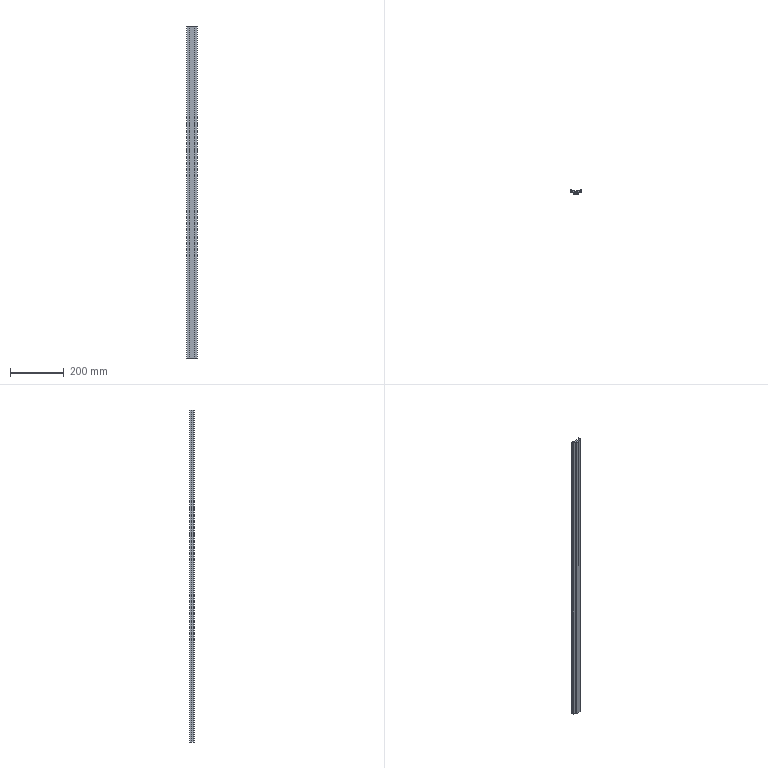Part | SolidWorks | features BaseBody 1 | 1 solid | 18 faces | box 38 x 15 x 1230 mm | volume 313896 mm3 | plane 18
STEP:
#1=CARTESIAN_POINT('',(-16.,11.5,1230.));
#2=VERTEX_POINT('',#1);
#3=CARTESIAN_POINT('',(-16.,11.5,0.));
#4=VERTEX_POINT('',#3);
#5=CARTESIAN_POINT('',(-16.,11.5,1230.));
#6=DIRECTION('',(0.,0.,-1.));
#7=VECTOR('',#6,1000.);
#8=LINE('',#5,#7);
#9=EDGE_CURVE('',#2,#4,#8,.T.);
#10=ORIENTED_EDGE('',*,*,#9,.F.);
#11=CARTESIAN_POINT('',(16.,11.5,1230.));
#12=VERTEX_POINT('',#11);
#13=CARTESIAN_POINT('',(16.,11.5,1230.));
#14=DIRECTION('',(-1.,0.,0.));
#15=VECTOR('',#14,1000.);
#16=LINE('',#13,#15);
#17=EDGE_CURVE('',#12,#2,#16,.T.);
#18=ORIENTED_EDGE('',*,*,#17,.F.);
#19=CARTESIAN_POINT('',(16.,11.5,0.));
#20=VERTEX_POINT('',#19);
#21=CARTESIAN_POINT('',(16.,11.5,1230.));
#22=DIRECTION('',(0.,0.,1.));
#23=VECTOR('',#22,1000.);
#24=LINE('',#21,#23);
#25=EDGE_CURVE('',#20,#12,#24,.T.);
#26=ORIENTED_EDGE('',*,*,#25,.F.);
#27=CARTESIAN_POINT('',(16.,11.5,0.));
#28=DIRECTION('',(1.,0.,0.));
#29=VECTOR('',#28,1000.);
#30=LINE('',#27,#29);
#31=EDGE_CURVE('',#4,#20,#30,.T.);
#32=ORIENTED_EDGE('',*,*,#31,.F.);
#33=EDGE_LOOP('',(#10,#18,#26,#32));
#34=FACE_OUTER_BOUND('',#33,.T.);
#35=CARTESIAN_POINT('',(16.,11.5,1230.));
#36=DIRECTION('',(0.,-1.,0.));
#37=DIRECTION('',(1.,0.,0.));
#38=AXIS2_PLACEMENT_3D('',#35,#36,#37);
#39=PLANE('',#38);
#40=ADVANCED_FACE('',(#34),#39,.F.);
#41=CARTESIAN_POINT('',(-3.5,3.,0.));
#42=VERTEX_POINT('',#41);
#43=CARTESIAN_POINT('',(-10.,3.,0.));
#44=VERTEX_POINT('',#43);
#45=CARTESIAN_POINT('',(0.,3.,0.));
#46=DIRECTION('',(-1.,0.,0.));
#47=VECTOR('',#46,1000.);
#48=LINE('',#45,#47);
#49=EDGE_CURVE('',#42,#44,#48,.T.);
#50=ORIENTED_EDGE('',*,*,#49,.F.);
#51=CARTESIAN_POINT('',(-3.5,7.8,0.));
#52=VERTEX_POINT('',#51);
#53=CARTESIAN_POINT('',(-3.5,0.,0.));
#54=DIRECTION('',(0.,-1.,0.));
#55=VECTOR('',#54,1000.);
#56=LINE('',#53,#55);
#57=EDGE_CURVE('',#52,#42,#56,.T.);
#58=ORIENTED_EDGE('',*,*,#57,.F.);
#59=CARTESIAN_POINT('',(-19.,7.8,0.));
#60=VERTEX_POINT('',#59);
#61=CARTESIAN_POINT('',(0.,7.8,0.));
#62=DIRECTION('',(1.,0.,0.));
#63=VECTOR('',#62,1000.);
#64=LINE('',#61,#63);
#65=EDGE_CURVE('',#60,#52,#64,.T.);
#66=ORIENTED_EDGE('',*,*,#65,.F.);
#67=CARTESIAN_POINT('',(-19.,15.,0.));
#68=VERTEX_POINT('',#67);
#69=CARTESIAN_POINT('',(-19.,0.,0.));
#70=DIRECTION('',(0.,-1.,0.));
#71=VECTOR('',#70,1000.);
#72=LINE('',#69,#71);
#73=EDGE_CURVE('',#68,#60,#72,.T.);
#74=ORIENTED_EDGE('',*,*,#73,.F.);
#75=CARTESIAN_POINT('',(-16.,15.,0.));
#76=VERTEX_POINT('',#75);
#77=CARTESIAN_POINT('',(0.,15.,0.));
#78=DIRECTION('',(-1.,0.,0.));
#79=VECTOR('',#78,1000.);
#80=LINE('',#77,#79);
#81=EDGE_CURVE('',#76,#68,#80,.T.);
#82=ORIENTED_EDGE('',*,*,#81,.F.);
#83=CARTESIAN_POINT('',(-16.,0.,0.));
#84=DIRECTION('',(0.,1.,0.));
#85=VECTOR('',#84,1000.);
#86=LINE('',#83,#85);
#87=EDGE_CURVE('',#4,#76,#86,.T.);
#88=ORIENTED_EDGE('',*,*,#87,.F.);
#89=ORIENTED_EDGE('',*,*,#31,.T.);
#90=CARTESIAN_POINT('',(16.,15.,0.));
#91=VERTEX_POINT('',#90);
#92=CARTESIAN_POINT('',(16.,0.,0.));
#93=DIRECTION('',(0.,-1.,0.));
#94=VECTOR('',#93,1000.);
#95=LINE('',#92,#94);
#96=EDGE_CURVE('',#91,#20,#95,.T.);
#97=ORIENTED_EDGE('',*,*,#96,.F.);
#98=CARTESIAN_POINT('',(19.,15.,0.));
#99=VERTEX_POINT('',#98);
#100=CARTESIAN_POINT('',(0.,15.,0.));
#101=DIRECTION('',(-1.,0.,0.));
#102=VECTOR('',#101,1000.);
#103=LINE('',#100,#102);
#104=EDGE_CURVE('',#99,#91,#103,.T.);
#105=ORIENTED_EDGE('',*,*,#104,.F.);
#106=CARTESIAN_POINT('',(19.,7.8,0.));
#107=VERTEX_POINT('',#106);
#108=CARTESIAN_POINT('',(19.,0.,0.));
#109=DIRECTION('',(0.,1.,0.));
#110=VECTOR('',#109,1000.);
#111=LINE('',#108,#110);
#112=EDGE_CURVE('',#107,#99,#111,.T.);
#113=ORIENTED_EDGE('',*,*,#112,.F.);
#114=CARTESIAN_POINT('',(3.5,7.8,0.));
#115=VERTEX_POINT('',#114);
#116=CARTESIAN_POINT('',(0.,7.8,0.));
#117=DIRECTION('',(1.,0.,0.));
#118=VECTOR('',#117,1000.);
#119=LINE('',#116,#118);
#120=EDGE_CURVE('',#115,#107,#119,.T.);
#121=ORIENTED_EDGE('',*,*,#120,.F.);
#122=CARTESIAN_POINT('',(3.5,3.,0.));
#123=VERTEX_POINT('',#122);
#124=CARTESIAN_POINT('',(3.5,0.,0.));
#125=DIRECTION('',(0.,1.,0.));
#126=VECTOR('',#125,1000.);
#127=LINE('',#124,#126);
#128=EDGE_CURVE('',#123,#115,#127,.T.);
#129=ORIENTED_EDGE('',*,*,#128,.F.);
#130=CARTESIAN_POINT('',(10.,3.,0.));
#131=VERTEX_POINT('',#130);
#132=CARTESIAN_POINT('',(0.,3.,0.));
#133=DIRECTION('',(-1.,0.,0.));
#134=VECTOR('',#133,1000.);
#135=LINE('',#132,#134);
#136=EDGE_CURVE('',#131,#123,#135,.T.);
#137=ORIENTED_EDGE('',*,*,#136,.F.);
#138=CARTESIAN_POINT('',(10.,0.,0.));
#139=VERTEX_POINT('',#138);
#140=CARTESIAN_POINT('',(10.,0.,0.));
#141=DIRECTION('',(0.,1.,0.));
#142=VECTOR('',#141,1000.);
#143=LINE('',#140,#142);
#144=EDGE_CURVE('',#139,#131,#143,.T.);
#145=ORIENTED_EDGE('',*,*,#144,.F.);
#146=CARTESIAN_POINT('',(-10.,0.,0.));
#147=VERTEX_POINT('',#146);
#148=CARTESIAN_POINT('',(0.,0.,0.));
#149=DIRECTION('',(1.,0.,0.));
#150=VECTOR('',#149,1000.);
#151=LINE('',#148,#150);
#152=EDGE_CURVE('',#147,#139,#151,.T.);
#153=ORIENTED_EDGE('',*,*,#152,.F.);
#154=CARTESIAN_POINT('',(-10.,0.,0.));
#155=DIRECTION('',(0.,-1.,0.));
#156=VECTOR('',#155,1000.);
#157=LINE('',#154,#156);
#158=EDGE_CURVE('',#44,#147,#157,.T.);
#159=ORIENTED_EDGE('',*,*,#158,.F.);
#160=EDGE_LOOP('',(#50,#58,#66,#74,#82,#88,#89,#97,#105,#113,#121,#129,#137,#145,#153,#159));
#161=FACE_OUTER_BOUND('',#160,.T.);
#162=CARTESIAN_POINT('',(0.,0.,0.));
#163=DIRECTION('',(0.,0.,1.));
#164=DIRECTION('',(1.,0.,0.));
#165=AXIS2_PLACEMENT_3D('',#162,#163,#164);
#166=PLANE('',#165);
#167=ADVANCED_FACE('',(#161),#166,.F.);
#168=CARTESIAN_POINT('',(-16.,15.,1230.));
#169=VERTEX_POINT('',#168);
#170=CARTESIAN_POINT('',(-16.,15.,1230.));
#171=DIRECTION('',(0.,0.,-1.));
#172=VECTOR('',#171,1000.);
#173=LINE('',#170,#172);
#174=EDGE_CURVE('',#169,#76,#173,.T.);
#175=ORIENTED_EDGE('',*,*,#174,.F.);
#176=CARTESIAN_POINT('',(-16.,11.5,1230.));
#177=DIRECTION('',(0.,1.,0.));
#178=VECTOR('',#177,1000.);
#179=LINE('',#176,#178);
#180=EDGE_CURVE('',#2,#169,#179,.T.);
#181=ORIENTED_EDGE('',*,*,#180,.F.);
#182=ORIENTED_EDGE('',*,*,#9,.T.);
#183=ORIENTED_EDGE('',*,*,#87,.T.);
#184=EDGE_LOOP('',(#175,#181,#182,#183));
#185=FACE_OUTER_BOUND('',#184,.T.);
#186=CARTESIAN_POINT('',(-16.,11.5,1230.));
#187=DIRECTION('',(-1.,0.,0.));
#188=DIRECTION('',(0.,-1.,0.));
#189=AXIS2_PLACEMENT_3D('',#186,#187,#188);
#190=PLANE('',#189);
#191=ADVANCED_FACE('',(#185),#190,.F.);
#192=CARTESIAN_POINT('',(-3.5,7.8,1230.));
#193=VERTEX_POINT('',#192);
#194=CARTESIAN_POINT('',(-3.5,3.,1230.));
#195=VERTEX_POINT('',#194);
#196=CARTESIAN_POINT('',(-3.5,0.,1230.));
#197=DIRECTION('',(0.,-1.,0.));
#198=VECTOR('',#197,1000.);
#199=LINE('',#196,#198);
#200=EDGE_CURVE('',#193,#195,#199,.T.);
#201=ORIENTED_EDGE('',*,*,#200,.T.);
#202=CARTESIAN_POINT('',(-10.,3.,1230.));
#203=VERTEX_POINT('',#202);
#204=CARTESIAN_POINT('',(0.,3.,1230.));
#205=DIRECTION('',(-1.,0.,0.));
#206=VECTOR('',#205,1000.);
#207=LINE('',#204,#206);
#208=EDGE_CURVE('',#195,#203,#207,.T.);
#209=ORIENTED_EDGE('',*,*,#208,.T.);
#210=CARTESIAN_POINT('',(-10.,0.,1230.));
#211=VERTEX_POINT('',#210);
#212=CARTESIAN_POINT('',(-10.,0.,1230.));
#213=DIRECTION('',(0.,-1.,0.));
#214=VECTOR('',#213,1000.);
#215=LINE('',#212,#214);
#216=EDGE_CURVE('',#203,#211,#215,.T.);
#217=ORIENTED_EDGE('',*,*,#216,.T.);
#218=CARTESIAN_POINT('',(10.,0.,1230.));
#219=VERTEX_POINT('',#218);
#220=CARTESIAN_POINT('',(0.,0.,1230.));
#221=DIRECTION('',(1.,0.,0.));
#222=VECTOR('',#221,1000.);
#223=LINE('',#220,#222);
#224=EDGE_CURVE('',#211,#219,#223,.T.);
#225=ORIENTED_EDGE('',*,*,#224,.T.);
#226=CARTESIAN_POINT('',(10.,3.,1230.));
#227=VERTEX_POINT('',#226);
#228=CARTESIAN_POINT('',(10.,0.,1230.));
#229=DIRECTION('',(0.,1.,0.));
#230=VECTOR('',#229,1000.);
#231=LINE('',#228,#230);
#232=EDGE_CURVE('',#219,#227,#231,.T.);
#233=ORIENTED_EDGE('',*,*,#232,.T.);
#234=CARTESIAN_POINT('',(3.5,3.,1230.));
#235=VERTEX_POINT('',#234);
#236=CARTESIAN_POINT('',(0.,3.,1230.));
#237=DIRECTION('',(-1.,0.,0.));
#238=VECTOR('',#237,1000.);
#239=LINE('',#236,#238);
#240=EDGE_CURVE('',#227,#235,#239,.T.);
#241=ORIENTED_EDGE('',*,*,#240,.T.);
#242=CARTESIAN_POINT('',(3.5,7.8,1230.));
#243=VERTEX_POINT('',#242);
#244=CARTESIAN_POINT('',(3.5,0.,1230.));
#245=DIRECTION('',(0.,1.,0.));
#246=VECTOR('',#245,1000.);
#247=LINE('',#244,#246);
#248=EDGE_CURVE('',#235,#243,#247,.T.);
#249=ORIENTED_EDGE('',*,*,#248,.T.);
#250=CARTESIAN_POINT('',(19.,7.8,1230.));
#251=VERTEX_POINT('',#250);
#252=CARTESIAN_POINT('',(0.,7.8,1230.));
#253=DIRECTION('',(1.,0.,0.));
#254=VECTOR('',#253,1000.);
#255=LINE('',#252,#254);
#256=EDGE_CURVE('',#243,#251,#255,.T.);
#257=ORIENTED_EDGE('',*,*,#256,.T.);
#258=CARTESIAN_POINT('',(19.,15.,1230.));
#259=VERTEX_POINT('',#258);
#260=CARTESIAN_POINT('',(19.,0.,1230.));
#261=DIRECTION('',(0.,1.,0.));
#262=VECTOR('',#261,1000.);
#263=LINE('',#260,#262);
#264=EDGE_CURVE('',#251,#259,#263,.T.);
#265=ORIENTED_EDGE('',*,*,#264,.T.);
#266=CARTESIAN_POINT('',(16.,15.,1230.));
#267=VERTEX_POINT('',#266);
#268=CARTESIAN_POINT('',(0.,15.,1230.));
#269=DIRECTION('',(-1.,0.,0.));
#270=VECTOR('',#269,1000.);
#271=LINE('',#268,#270);
#272=EDGE_CURVE('',#259,#267,#271,.T.);
#273=ORIENTED_EDGE('',*,*,#272,.T.);
#274=CARTESIAN_POINT('',(16.,0.,1230.));
#275=DIRECTION('',(0.,-1.,0.));
#276=VECTOR('',#275,1000.);
#277=LINE('',#274,#276);
#278=EDGE_CURVE('',#267,#12,#277,.T.);
#279=ORIENTED_EDGE('',*,*,#278,.T.);
#280=ORIENTED_EDGE('',*,*,#17,.T.);
#281=ORIENTED_EDGE('',*,*,#180,.T.);
#282=CARTESIAN_POINT('',(-19.,15.,1230.));
#283=VERTEX_POINT('',#282);
#284=CARTESIAN_POINT('',(0.,15.,1230.));
#285=DIRECTION('',(-1.,0.,0.));
#286=VECTOR('',#285,1000.);
#287=LINE('',#284,#286);
#288=EDGE_CURVE('',#169,#283,#287,.T.);
#289=ORIENTED_EDGE('',*,*,#288,.T.);
#290=CARTESIAN_POINT('',(-19.,7.8,1230.));
#291=VERTEX_POINT('',#290);
#292=CARTESIAN_POINT('',(-19.,0.,1230.));
#293=DIRECTION('',(0.,-1.,0.));
#294=VECTOR('',#293,1000.);
#295=LINE('',#292,#294);
#296=EDGE_CURVE('',#283,#291,#295,.T.);
#297=ORIENTED_EDGE('',*,*,#296,.T.);
#298=CARTESIAN_POINT('',(0.,7.8,1230.));
#299=DIRECTION('',(1.,0.,0.));
#300=VECTOR('',#299,1000.);
#301=LINE('',#298,#300);
#302=EDGE_CURVE('',#291,#193,#301,.T.);
#303=ORIENTED_EDGE('',*,*,#302,.T.);
#304=EDGE_LOOP('',(#201,#209,#217,#225,#233,#241,#249,#257,#265,#273,#279,#280,#281,#289,#297,#303));
#305=FACE_OUTER_BOUND('',#304,.T.);
#306=CARTESIAN_POINT('',(0.,0.,1230.));
#307=DIRECTION('',(0.,0.,1.));
#308=DIRECTION('',(1.,0.,0.));
#309=AXIS2_PLACEMENT_3D('',#306,#307,#308);
#310=PLANE('',#309);
#311=ADVANCED_FACE('',(#305),#310,.T.);
#312=ORIENTED_EDGE('',*,*,#25,.T.);
#313=ORIENTED_EDGE('',*,*,#278,.F.);
#314=CARTESIAN_POINT('',(16.,15.,1230.));
#315=DIRECTION('',(0.,0.,1.));
#316=VECTOR('',#315,1000.);
#317=LINE('',#314,#316);
#318=EDGE_CURVE('',#91,#267,#317,.T.);
#319=ORIENTED_EDGE('',*,*,#318,.F.);
#320=ORIENTED_EDGE('',*,*,#96,.T.);
#321=EDGE_LOOP('',(#312,#313,#319,#320));
#322=FACE_OUTER_BOUND('',#321,.T.);
#323=CARTESIAN_POINT('',(16.,15.,1230.));
#324=DIRECTION('',(1.,0.,0.));
#325=DIRECTION('',(0.,1.,0.));
#326=AXIS2_PLACEMENT_3D('',#323,#324,#325);
#327=PLANE('',#326);
#328=ADVANCED_FACE('',(#322),#327,.F.);
#329=CARTESIAN_POINT('',(-10.,0.,1230.));
#330=DIRECTION('',(0.,0.,-1.));
#331=VECTOR('',#330,1000.);
#332=LINE('',#329,#331);
#333=EDGE_CURVE('',#211,#147,#332,.T.);
#334=ORIENTED_EDGE('',*,*,#333,.F.);
#335=ORIENTED_EDGE('',*,*,#216,.F.);
#336=CARTESIAN_POINT('',(-10.,3.,1230.));
#337=DIRECTION('',(0.,0.,1.));
#338=VECTOR('',#337,1000.);
#339=LINE('',#336,#338);
#340=EDGE_CURVE('',#44,#203,#339,.T.);
#341=ORIENTED_EDGE('',*,*,#340,.F.);
#342=ORIENTED_EDGE('',*,*,#158,.T.);
#343=EDGE_LOOP('',(#334,#335,#341,#342));
#344=FACE_OUTER_BOUND('',#343,.T.);
#345=CARTESIAN_POINT('',(-10.,3.,1230.));
#346=DIRECTION('',(1.,0.,0.));
#347=DIRECTION('',(0.,0.,-1.));
#348=AXIS2_PLACEMENT_3D('',#345,#346,#347);
#349=PLANE('',#348);
#350=ADVANCED_FACE('',(#344),#349,.F.);
#351=ORIENTED_EDGE('',*,*,#340,.T.);
#352=ORIENTED_EDGE('',*,*,#208,.F.);
#353=CARTESIAN_POINT('',(-3.5,3.,1230.));
#354=DIRECTION('',(0.,0.,1.));
#355=VECTOR('',#354,1000.);
#356=LINE('',#353,#355);
#357=EDGE_CURVE('',#42,#195,#356,.T.);
#358=ORIENTED_EDGE('',*,*,#357,.F.);
#359=ORIENTED_EDGE('',*,*,#49,.T.);
#360=EDGE_LOOP('',(#351,#352,#358,#359));
#361=FACE_OUTER_BOUND('',#360,.T.);
#362=CARTESIAN_POINT('',(-3.5,3.,1230.));
#363=DIRECTION('',(0.,-1.,0.));
#364=DIRECTION('',(1.,0.,0.));
#365=AXIS2_PLACEMENT_3D('',#362,#363,#364);
#366=PLANE('',#365);
#367=ADVANCED_FACE('',(#361),#366,.F.);
#368=ORIENTED_EDGE('',*,*,#357,.T.);
#369=ORIENTED_EDGE('',*,*,#200,.F.);
#370=CARTESIAN_POINT('',(-3.5,7.8,1230.));
#371=DIRECTION('',(0.,0.,1.));
#372=VECTOR('',#371,1000.);
#373=LINE('',#370,#372);
#374=EDGE_CURVE('',#52,#193,#373,.T.);
#375=ORIENTED_EDGE('',*,*,#374,.F.);
#376=ORIENTED_EDGE('',*,*,#57,.T.);
#377=EDGE_LOOP('',(#368,#369,#375,#376));
#378=FACE_OUTER_BOUND('',#377,.T.);
#379=CARTESIAN_POINT('',(-3.5,7.8,1230.));
#380=DIRECTION('',(1.,0.,0.));
#381=DIRECTION('',(0.,1.,0.));
#382=AXIS2_PLACEMENT_3D('',#379,#380,#381);
#383=PLANE('',#382);
#384=ADVANCED_FACE('',(#378),#383,.F.);
#385=ORIENTED_EDGE('',*,*,#374,.T.);
#386=ORIENTED_EDGE('',*,*,#302,.F.);
#387=CARTESIAN_POINT('',(-19.,7.8,1230.));
#388=DIRECTION('',(0.,0.,1.));
#389=VECTOR('',#388,1000.);
#390=LINE('',#387,#389);
#391=EDGE_CURVE('',#60,#291,#390,.T.);
#392=ORIENTED_EDGE('',*,*,#391,.F.);
#393=ORIENTED_EDGE('',*,*,#65,.T.);
#394=EDGE_LOOP('',(#385,#386,#392,#393));
#395=FACE_OUTER_BOUND('',#394,.T.);
#396=CARTESIAN_POINT('',(-19.,7.8,1230.));
#397=DIRECTION('',(0.,1.,0.));
#398=DIRECTION('',(0.,0.,1.));
#399=AXIS2_PLACEMENT_3D('',#396,#397,#398);
#400=PLANE('',#399);
#401=ADVANCED_FACE('',(#395),#400,.F.);
#402=ORIENTED_EDGE('',*,*,#391,.T.);
#403=ORIENTED_EDGE('',*,*,#296,.F.);
#404=CARTESIAN_POINT('',(-19.,15.,1230.));
#405=DIRECTION('',(0.,0.,1.));
#406=VECTOR('',#405,1000.);
#407=LINE('',#404,#406);
#408=EDGE_CURVE('',#68,#283,#407,.T.);
#409=ORIENTED_EDGE('',*,*,#408,.F.);
#410=ORIENTED_EDGE('',*,*,#73,.T.);
#411=EDGE_LOOP('',(#402,#403,#409,#410));
#412=FACE_OUTER_BOUND('',#411,.T.);
#413=CARTESIAN_POINT('',(-19.,15.,1230.));
#414=DIRECTION('',(1.,0.,0.));
#415=DIRECTION('',(0.,1.,0.));
#416=AXIS2_PLACEMENT_3D('',#413,#414,#415);
#417=PLANE('',#416);
#418=ADVANCED_FACE('',(#412),#417,.F.);
#419=ORIENTED_EDGE('',*,*,#408,.T.);
#420=ORIENTED_EDGE('',*,*,#288,.F.);
#421=ORIENTED_EDGE('',*,*,#174,.T.);
#422=ORIENTED_EDGE('',*,*,#81,.T.);
#423=EDGE_LOOP('',(#419,#420,#421,#422));
#424=FACE_OUTER_BOUND('',#423,.T.);
#425=CARTESIAN_POINT('',(-16.,15.,1230.));
#426=DIRECTION('',(0.,-1.,0.));
#427=DIRECTION('',(0.,0.,-1.));
#428=AXIS2_PLACEMENT_3D('',#425,#426,#427);
#429=PLANE('',#428);
#430=ADVANCED_FACE('',(#424),#429,.F.);
#431=ORIENTED_EDGE('',*,*,#318,.T.);
#432=ORIENTED_EDGE('',*,*,#272,.F.);
#433=CARTESIAN_POINT('',(19.,15.,1230.));
#434=DIRECTION('',(0.,0.,1.));
#435=VECTOR('',#434,1000.);
#436=LINE('',#433,#435);
#437=EDGE_CURVE('',#99,#259,#436,.T.);
#438=ORIENTED_EDGE('',*,*,#437,.F.);
#439=ORIENTED_EDGE('',*,*,#104,.T.);
#440=EDGE_LOOP('',(#431,#432,#438,#439));
#441=FACE_OUTER_BOUND('',#440,.T.);
#442=CARTESIAN_POINT('',(19.,15.,1230.));
#443=DIRECTION('',(0.,-1.,0.));
#444=DIRECTION('',(1.,0.,0.));
#445=AXIS2_PLACEMENT_3D('',#442,#443,#444);
#446=PLANE('',#445);
#447=ADVANCED_FACE('',(#441),#446,.F.);
#448=ORIENTED_EDGE('',*,*,#437,.T.);
#449=ORIENTED_EDGE('',*,*,#264,.F.);
#450=CARTESIAN_POINT('',(19.,7.8,1230.));
#451=DIRECTION('',(0.,0.,1.));
#452=VECTOR('',#451,1000.);
#453=LINE('',#450,#452);
#454=EDGE_CURVE('',#107,#251,#453,.T.);
#455=ORIENTED_EDGE('',*,*,#454,.F.);
#456=ORIENTED_EDGE('',*,*,#112,.T.);
#457=EDGE_LOOP('',(#448,#449,#455,#456));
#458=FACE_OUTER_BOUND('',#457,.T.);
#459=CARTESIAN_POINT('',(19.,7.8,1230.));
#460=DIRECTION('',(-1.,0.,0.));
#461=DIRECTION('',(0.,-1.,0.));
#462=AXIS2_PLACEMENT_3D('',#459,#460,#461);
#463=PLANE('',#462);
#464=ADVANCED_FACE('',(#458),#463,.F.);
#465=ORIENTED_EDGE('',*,*,#454,.T.);
#466=ORIENTED_EDGE('',*,*,#256,.F.);
#467=CARTESIAN_POINT('',(3.5,7.8,1230.));
#468=DIRECTION('',(0.,0.,1.));
#469=VECTOR('',#468,1000.);
#470=LINE('',#467,#469);
#471=EDGE_CURVE('',#115,#243,#470,.T.);
#472=ORIENTED_EDGE('',*,*,#471,.F.);
#473=ORIENTED_EDGE('',*,*,#120,.T.);
#474=EDGE_LOOP('',(#465,#466,#472,#473));
#475=FACE_OUTER_BOUND('',#474,.T.);
#476=CARTESIAN_POINT('',(3.5,7.8,1230.));
#477=DIRECTION('',(0.,1.,0.));
#478=DIRECTION('',(-1.,0.,0.));
#479=AXIS2_PLACEMENT_3D('',#476,#477,#478);
#480=PLANE('',#479);
#481=ADVANCED_FACE('',(#475),#480,.F.);
#482=ORIENTED_EDGE('',*,*,#471,.T.);
#483=ORIENTED_EDGE('',*,*,#248,.F.);
#484=CARTESIAN_POINT('',(3.5,3.,1230.));
#485=DIRECTION('',(0.,0.,1.));
#486=VECTOR('',#485,1000.);
#487=LINE('',#484,#486);
#488=EDGE_CURVE('',#123,#235,#487,.T.);
#489=ORIENTED_EDGE('',*,*,#488,.F.);
#490=ORIENTED_EDGE('',*,*,#128,.T.);
#491=EDGE_LOOP('',(#482,#483,#489,#490));
#492=FACE_OUTER_BOUND('',#491,.T.);
#493=CARTESIAN_POINT('',(3.5,3.,1230.));
#494=DIRECTION('',(-1.,0.,0.));
#495=DIRECTION('',(0.,0.,1.));
#496=AXIS2_PLACEMENT_3D('',#493,#494,#495);
#497=PLANE('',#496);
#498=ADVANCED_FACE('',(#492),#497,.F.);
#499=ORIENTED_EDGE('',*,*,#488,.T.);
#500=ORIENTED_EDGE('',*,*,#240,.F.);
#501=CARTESIAN_POINT('',(10.,3.,1230.));
#502=DIRECTION('',(0.,0.,1.));
#503=VECTOR('',#502,1000.);
#504=LINE('',#501,#503);
#505=EDGE_CURVE('',#131,#227,#504,.T.);
#506=ORIENTED_EDGE('',*,*,#505,.F.);
#507=ORIENTED_EDGE('',*,*,#136,.T.);
#508=EDGE_LOOP('',(#499,#500,#506,#507));
#509=FACE_OUTER_BOUND('',#508,.T.);
#510=CARTESIAN_POINT('',(10.,3.,1230.));
#511=DIRECTION('',(0.,-1.,0.));
#512=DIRECTION('',(1.,0.,0.));
#513=AXIS2_PLACEMENT_3D('',#510,#511,#512);
#514=PLANE('',#513);
#515=ADVANCED_FACE('',(#509),#514,.F.);
#516=ORIENTED_EDGE('',*,*,#505,.T.);
#517=ORIENTED_EDGE('',*,*,#232,.F.);
#518=CARTESIAN_POINT('',(10.,0.,1230.));
#519=DIRECTION('',(0.,0.,1.));
#520=VECTOR('',#519,1000.);
#521=LINE('',#518,#520);
#522=EDGE_CURVE('',#139,#219,#521,.T.);
#523=ORIENTED_EDGE('',*,*,#522,.F.);
#524=ORIENTED_EDGE('',*,*,#144,.T.);
#525=EDGE_LOOP('',(#516,#517,#523,#524));
#526=FACE_OUTER_BOUND('',#525,.T.);
#527=CARTESIAN_POINT('',(10.,0.,1230.));
#528=DIRECTION('',(-1.,0.,0.));
#529=DIRECTION('',(0.,-1.,0.));
#530=AXIS2_PLACEMENT_3D('',#527,#528,#529);
#531=PLANE('',#530);
#532=ADVANCED_FACE('',(#526),#531,.F.);
#533=ORIENTED_EDGE('',*,*,#522,.T.);
#534=ORIENTED_EDGE('',*,*,#224,.F.);
#535=ORIENTED_EDGE('',*,*,#333,.T.);
#536=ORIENTED_EDGE('',*,*,#152,.T.);
#537=EDGE_LOOP('',(#533,#534,#535,#536));
#538=FACE_OUTER_BOUND('',#537,.T.);
#539=CARTESIAN_POINT('',(-10.,0.,1230.));
#540=DIRECTION('',(0.,1.,0.));
#541=DIRECTION('',(-1.,0.,0.));
#542=AXIS2_PLACEMENT_3D('',#539,#540,#541);
#543=PLANE('',#542);
#544=ADVANCED_FACE('',(#538),#543,.F.);
#545=CLOSED_SHELL('',(#40,#167,#191,#311,#328,#350,#367,#384,#401,#418,#430,#447,#464,#481,#498,#515,#532,#544));
#546=MANIFOLD_SOLID_BREP('',#545);
#547=CARTESIAN_POINT('',(0.,0.,0.));
#548=DIRECTION('',(0.,0.,1.));
#549=DIRECTION('',(1.,0.,0.));
#550=AXIS2_PLACEMENT_3D('',#547,#548,#549);
#551=(LENGTH_UNIT()NAMED_UNIT(*)SI_UNIT(.MILLI.,.METRE.));
#552=UNCERTAINTY_MEASURE_WITH_UNIT(LENGTH_MEASURE(0.00001),#551,'','');
#553=(NAMED_UNIT(*)PLANE_ANGLE_UNIT()SI_UNIT($,.RADIAN.));
#554=(NAMED_UNIT(*)SI_UNIT($,.STERADIAN.)SOLID_ANGLE_UNIT());
#555=(GEOMETRIC_REPRESENTATION_CONTEXT(3)GLOBAL_UNCERTAINTY_ASSIGNED_CONTEXT((#552))GLOBAL_UNIT_ASSIGNED_CONTEXT((#551,#553,#554))REPRESENTATION_CONTEXT('',''));
#556=ADVANCED_BREP_SHAPE_REPRESENTATION('',(#546,#550),#555);